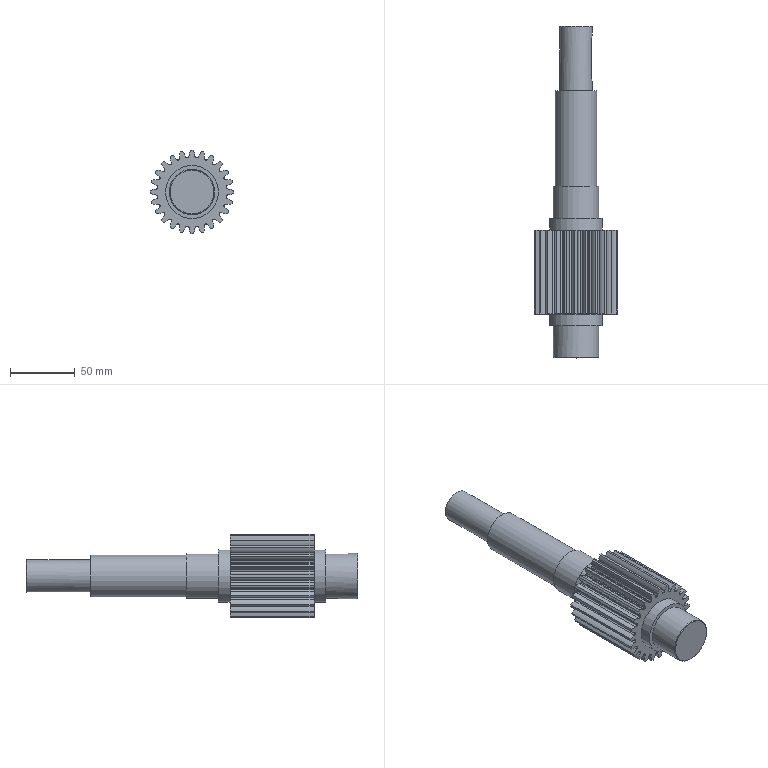Part | NX | features BREP 24, META 24, DATUM_CSYS 8, EXTRUDE 7, SKETCH 7, EXTRACT_DATUM_AXIS 4, EXTRACT_DATUM_PLANE 2, EXTRACT_STRING 2, BLEND 1, CHAMFER 1, CYLINDER 1, FSET 1, Instance Feature 1, Mirror Feature 1 | 1 solid | 165 faces | box 65 x 257 x 65 mm | volume 335559 mm3 | spline 120 | cylinder 32 | plane 11 | cone 2 | commonest cylinder face diameters 53.75 x24 8 x2 35 x2 41 x2 25 x1 32 x1